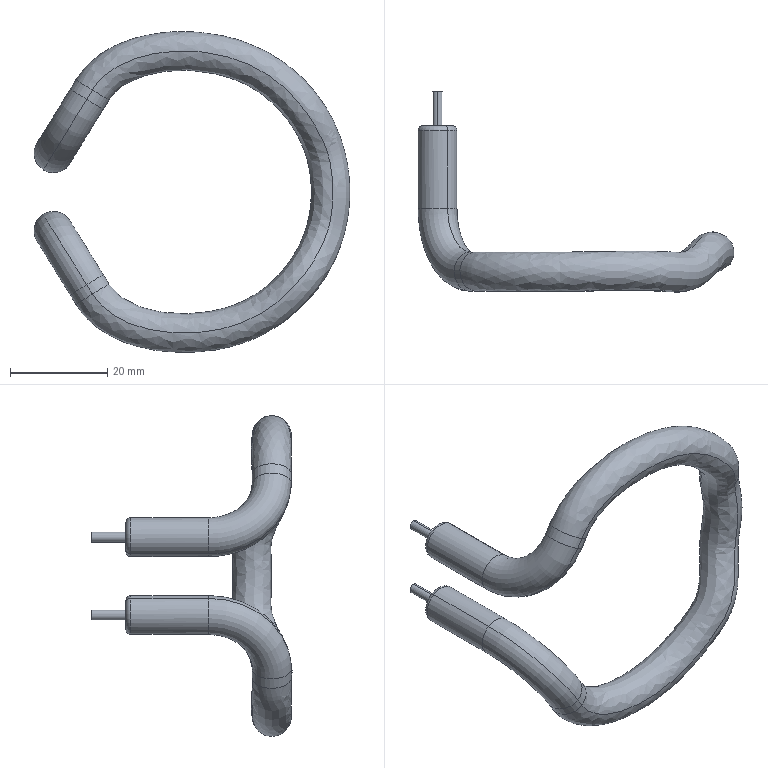Part | STEP file | JIAREIGUAN_56_1 | 1 solid | 26 faces | box 65 x 41.193 x 66.044 mm | volume 10951 mm3 | cylinder 12 | torus 8 | plane 4 | spline 2 | commonest cylinder face diameters 8 x8 2 x4